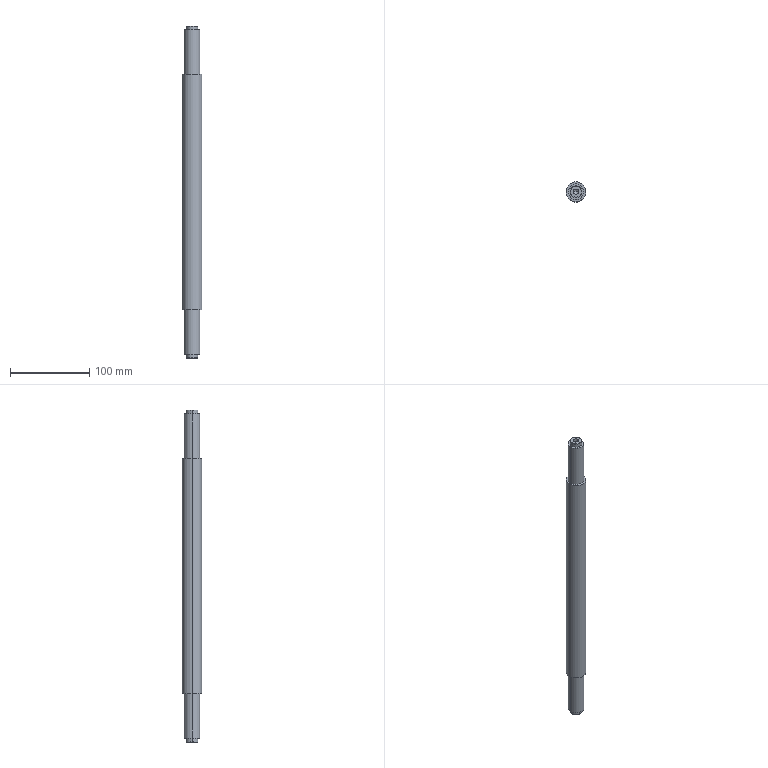Part | SolidWorks | features ICE 4, Chamfer 2, HoleWzd 2, Extrusion 1 | 1 solid | 28 faces | box 25 x 25 x 420 mm | volume 181738 mm3 | cylinder 14 | cone 8 | plane 6 | commonest cylinder face diameters 6.8 x4 15 x4 20 x4 25 x2
STEP:
#1=CARTESIAN_POINT('',(-7.,0.,-61.));
#2=VERTEX_POINT('',#1);
#3=CARTESIAN_POINT('',(7.,0.,-61.));
#4=VERTEX_POINT('',#3);
#5=CARTESIAN_POINT('',(0.,0.,-61.));
#6=DIRECTION('',(0.,0.,-1.));
#7=DIRECTION('',(-1.,0.,0.));
#8=AXIS2_PLACEMENT_3D('',#5,#6,#7);
#9=CIRCLE('',#8,7.);
#10=EDGE_CURVE('',#2,#4,#9,.T.);
#11=ORIENTED_EDGE('',*,*,#10,.F.);
#12=CARTESIAN_POINT('',(-7.5,0.,-60.5));
#13=VERTEX_POINT('',#12);
#14=CARTESIAN_POINT('',(-7.,0.,-61.));
#15=DIRECTION('',(-0.7071,0.,0.7071));
#16=VECTOR('',#15,1000.);
#17=LINE('',#14,#16);
#18=EDGE_CURVE('',#2,#13,#17,.T.);
#19=ORIENTED_EDGE('',*,*,#18,.T.);
#20=CARTESIAN_POINT('',(7.5,0.,-60.5));
#21=VERTEX_POINT('',#20);
#22=CARTESIAN_POINT('',(0.,0.,-60.5));
#23=DIRECTION('',(0.,0.,1.));
#24=DIRECTION('',(-1.,0.,0.));
#25=AXIS2_PLACEMENT_3D('',#22,#23,#24);
#26=CIRCLE('',#25,7.5);
#27=EDGE_CURVE('',#21,#13,#26,.T.);
#28=ORIENTED_EDGE('',*,*,#27,.F.);
#29=CARTESIAN_POINT('',(7.,0.,-61.));
#30=DIRECTION('',(0.7071,0.,0.7071));
#31=VECTOR('',#30,1000.);
#32=LINE('',#29,#31);
#33=EDGE_CURVE('',#4,#21,#32,.T.);
#34=ORIENTED_EDGE('',*,*,#33,.F.);
#35=EDGE_LOOP('',(#11,#19,#28,#34));
#36=FACE_OUTER_BOUND('',#35,.T.);
#37=CARTESIAN_POINT('',(0.,0.,-61.));
#38=DIRECTION('',(0.,0.,1.));
#39=DIRECTION('',(1.,0.,0.));
#40=AXIS2_PLACEMENT_3D('',#37,#38,#39);
#41=CONICAL_SURFACE('',#40,7.,0.7854);
#42=ADVANCED_FACE('',(#36),#41,.T.);
#43=CARTESIAN_POINT('',(7.,0.,359.));
#44=VERTEX_POINT('',#43);
#45=CARTESIAN_POINT('',(-7.,0.,359.));
#46=VERTEX_POINT('',#45);
#47=CARTESIAN_POINT('',(0.,0.,359.));
#48=DIRECTION('',(0.,0.,1.));
#49=DIRECTION('',(1.,0.,0.));
#50=AXIS2_PLACEMENT_3D('',#47,#48,#49);
#51=CIRCLE('',#50,7.);
#52=EDGE_CURVE('',#44,#46,#51,.T.);
#53=ORIENTED_EDGE('',*,*,#52,.F.);
#54=CARTESIAN_POINT('',(7.5,0.,358.5));
#55=VERTEX_POINT('',#54);
#56=CARTESIAN_POINT('',(7.,0.,359.));
#57=DIRECTION('',(0.7071,0.,-0.7071));
#58=VECTOR('',#57,1000.);
#59=LINE('',#56,#58);
#60=EDGE_CURVE('',#44,#55,#59,.T.);
#61=ORIENTED_EDGE('',*,*,#60,.T.);
#62=CARTESIAN_POINT('',(-7.5,0.,358.5));
#63=VERTEX_POINT('',#62);
#64=CARTESIAN_POINT('',(0.,0.,358.5));
#65=DIRECTION('',(0.,0.,-1.));
#66=DIRECTION('',(1.,0.,0.));
#67=AXIS2_PLACEMENT_3D('',#64,#65,#66);
#68=CIRCLE('',#67,7.5);
#69=EDGE_CURVE('',#63,#55,#68,.T.);
#70=ORIENTED_EDGE('',*,*,#69,.F.);
#71=CARTESIAN_POINT('',(-7.,0.,359.));
#72=DIRECTION('',(-0.7071,0.,-0.7071));
#73=VECTOR('',#72,1000.);
#74=LINE('',#71,#73);
#75=EDGE_CURVE('',#46,#63,#74,.T.);
#76=ORIENTED_EDGE('',*,*,#75,.F.);
#77=EDGE_LOOP('',(#53,#61,#70,#76));
#78=FACE_OUTER_BOUND('',#77,.T.);
#79=CARTESIAN_POINT('',(0.,0.,359.));
#80=DIRECTION('',(0.,0.,-1.));
#81=DIRECTION('',(-1.,0.,0.));
#82=AXIS2_PLACEMENT_3D('',#79,#80,#81);
#83=CONICAL_SURFACE('',#82,7.,0.7854);
#84=ADVANCED_FACE('',(#78),#83,.T.);
#85=CARTESIAN_POINT('',(-3.4,0.,339.25));
#86=VERTEX_POINT('',#85);
#87=CARTESIAN_POINT('',(3.4,0.,339.25));
#88=VERTEX_POINT('',#87);
#89=CARTESIAN_POINT('',(0.,0.,339.25));
#90=DIRECTION('',(0.,0.,1.));
#91=DIRECTION('',(1.,0.,0.));
#92=AXIS2_PLACEMENT_3D('',#89,#90,#91);
#93=CIRCLE('',#92,3.4);
#94=EDGE_CURVE('',#86,#88,#93,.T.);
#95=ORIENTED_EDGE('',*,*,#94,.F.);
#96=CARTESIAN_POINT('',(-3.4,0.,359.));
#97=VERTEX_POINT('',#96);
#98=CARTESIAN_POINT('',(-3.4,0.,359.));
#99=DIRECTION('',(0.,0.,1.));
#100=VECTOR('',#99,1000.);
#101=LINE('',#98,#100);
#102=EDGE_CURVE('',#86,#97,#101,.T.);
#103=ORIENTED_EDGE('',*,*,#102,.T.);
#104=CARTESIAN_POINT('',(3.4,0.,359.));
#105=VERTEX_POINT('',#104);
#106=CARTESIAN_POINT('',(0.,0.,359.));
#107=DIRECTION('',(0.,0.,1.));
#108=DIRECTION('',(1.,0.,0.));
#109=AXIS2_PLACEMENT_3D('',#106,#107,#108);
#110=CIRCLE('',#109,3.4);
#111=EDGE_CURVE('',#97,#105,#110,.T.);
#112=ORIENTED_EDGE('',*,*,#111,.T.);
#113=CARTESIAN_POINT('',(3.4,0.,359.));
#114=DIRECTION('',(0.,0.,1.));
#115=VECTOR('',#114,1000.);
#116=LINE('',#113,#115);
#117=EDGE_CURVE('',#88,#105,#116,.T.);
#118=ORIENTED_EDGE('',*,*,#117,.F.);
#119=EDGE_LOOP('',(#95,#103,#112,#118));
#120=FACE_OUTER_BOUND('',#119,.T.);
#121=CARTESIAN_POINT('',(0.,0.,359.));
#122=DIRECTION('',(0.,0.,1.));
#123=DIRECTION('',(1.,0.,0.));
#124=AXIS2_PLACEMENT_3D('',#121,#122,#123);
#125=CYLINDRICAL_SURFACE('',#124,3.4);
#126=ADVANCED_FACE('',(#120),#125,.F.);
#127=CARTESIAN_POINT('',(0.,0.,337.207));
#128=VERTEX_POINT('',#127);
#129=CARTESIAN_POINT('',(3.4,0.,339.25));
#130=DIRECTION('',(0.8572,0.,0.515));
#131=VECTOR('',#130,1000.);
#132=LINE('',#129,#131);
#133=EDGE_CURVE('',#128,#88,#132,.T.);
#134=ORIENTED_EDGE('',*,*,#133,.F.);
#135=CARTESIAN_POINT('',(-3.4,0.,339.25));
#136=DIRECTION('',(-0.8572,0.,0.515));
#137=VECTOR('',#136,1000.);
#138=LINE('',#135,#137);
#139=EDGE_CURVE('',#128,#86,#138,.T.);
#140=ORIENTED_EDGE('',*,*,#139,.T.);
#141=ORIENTED_EDGE('',*,*,#94,.T.);
#142=EDGE_LOOP('',(#134,#140,#141));
#143=FACE_OUTER_BOUND('',#142,.T.);
#144=CARTESIAN_POINT('',(0.,0.,339.25));
#145=DIRECTION('',(0.,0.,1.));
#146=DIRECTION('',(1.,0.,0.));
#147=AXIS2_PLACEMENT_3D('',#144,#145,#146);
#148=CONICAL_SURFACE('',#147,3.4,1.03);
#149=ADVANCED_FACE('',(#143),#148,.F.);
#150=CARTESIAN_POINT('',(3.4,0.,-41.25));
#151=VERTEX_POINT('',#150);
#152=CARTESIAN_POINT('',(-3.4,0.,-41.25));
#153=VERTEX_POINT('',#152);
#154=CARTESIAN_POINT('',(0.,0.,-41.25));
#155=DIRECTION('',(0.,0.,-1.));
#156=DIRECTION('',(-1.,0.,0.));
#157=AXIS2_PLACEMENT_3D('',#154,#155,#156);
#158=CIRCLE('',#157,3.4);
#159=EDGE_CURVE('',#151,#153,#158,.T.);
#160=ORIENTED_EDGE('',*,*,#159,.F.);
#161=CARTESIAN_POINT('',(3.4,0.,-61.));
#162=VERTEX_POINT('',#161);
#163=CARTESIAN_POINT('',(3.4,0.,-61.));
#164=DIRECTION('',(0.,0.,-1.));
#165=VECTOR('',#164,1000.);
#166=LINE('',#163,#165);
#167=EDGE_CURVE('',#151,#162,#166,.T.);
#168=ORIENTED_EDGE('',*,*,#167,.T.);
#169=CARTESIAN_POINT('',(-3.4,0.,-61.));
#170=VERTEX_POINT('',#169);
#171=CARTESIAN_POINT('',(0.,0.,-61.));
#172=DIRECTION('',(0.,0.,-1.));
#173=DIRECTION('',(-1.,0.,0.));
#174=AXIS2_PLACEMENT_3D('',#171,#172,#173);
#175=CIRCLE('',#174,3.4);
#176=EDGE_CURVE('',#162,#170,#175,.T.);
#177=ORIENTED_EDGE('',*,*,#176,.T.);
#178=CARTESIAN_POINT('',(-3.4,0.,-61.));
#179=DIRECTION('',(0.,0.,-1.));
#180=VECTOR('',#179,1000.);
#181=LINE('',#178,#180);
#182=EDGE_CURVE('',#153,#170,#181,.T.);
#183=ORIENTED_EDGE('',*,*,#182,.F.);
#184=EDGE_LOOP('',(#160,#168,#177,#183));
#185=FACE_OUTER_BOUND('',#184,.T.);
#186=CARTESIAN_POINT('',(0.,0.,-61.));
#187=DIRECTION('',(0.,0.,-1.));
#188=DIRECTION('',(-1.,0.,0.));
#189=AXIS2_PLACEMENT_3D('',#186,#187,#188);
#190=CYLINDRICAL_SURFACE('',#189,3.4);
#191=ADVANCED_FACE('',(#185),#190,.F.);
#192=CARTESIAN_POINT('',(0.,0.,-39.207));
#193=VERTEX_POINT('',#192);
#194=CARTESIAN_POINT('',(-3.4,0.,-41.25));
#195=DIRECTION('',(-0.8572,0.,-0.515));
#196=VECTOR('',#195,1000.);
#197=LINE('',#194,#196);
#198=EDGE_CURVE('',#193,#153,#197,.T.);
#199=ORIENTED_EDGE('',*,*,#198,.F.);
#200=CARTESIAN_POINT('',(3.4,0.,-41.25));
#201=DIRECTION('',(0.8572,0.,-0.515));
#202=VECTOR('',#201,1000.);
#203=LINE('',#200,#202);
#204=EDGE_CURVE('',#193,#151,#203,.T.);
#205=ORIENTED_EDGE('',*,*,#204,.T.);
#206=ORIENTED_EDGE('',*,*,#159,.T.);
#207=EDGE_LOOP('',(#199,#205,#206));
#208=FACE_OUTER_BOUND('',#207,.T.);
#209=CARTESIAN_POINT('',(0.,0.,-41.25));
#210=DIRECTION('',(0.,0.,-1.));
#211=DIRECTION('',(-1.,0.,0.));
#212=AXIS2_PLACEMENT_3D('',#209,#210,#211);
#213=CONICAL_SURFACE('',#212,3.4,1.03);
#214=ADVANCED_FACE('',(#208),#213,.F.);
#215=ORIENTED_EDGE('',*,*,#27,.T.);
#216=CARTESIAN_POINT('',(-7.5,0.,-56.));
#217=VERTEX_POINT('',#216);
#218=CARTESIAN_POINT('',(-7.5,0.,-61.));
#219=DIRECTION('',(0.,0.,1.));
#220=VECTOR('',#219,1000.);
#221=LINE('',#218,#220);
#222=EDGE_CURVE('',#13,#217,#221,.T.);
#223=ORIENTED_EDGE('',*,*,#222,.T.);
#224=CARTESIAN_POINT('',(7.5,0.,-56.));
#225=VERTEX_POINT('',#224);
#226=CARTESIAN_POINT('',(0.,0.,-56.));
#227=DIRECTION('',(0.,0.,-1.));
#228=DIRECTION('',(-1.,0.,0.));
#229=AXIS2_PLACEMENT_3D('',#226,#227,#228);
#230=CIRCLE('',#229,7.5);
#231=EDGE_CURVE('',#217,#225,#230,.T.);
#232=ORIENTED_EDGE('',*,*,#231,.T.);
#233=CARTESIAN_POINT('',(7.5,0.,-61.));
#234=DIRECTION('',(0.,0.,1.));
#235=VECTOR('',#234,1000.);
#236=LINE('',#233,#235);
#237=EDGE_CURVE('',#21,#225,#236,.T.);
#238=ORIENTED_EDGE('',*,*,#237,.F.);
#239=EDGE_LOOP('',(#215,#223,#232,#238));
#240=FACE_OUTER_BOUND('',#239,.T.);
#241=CARTESIAN_POINT('',(0.,0.,-61.));
#242=DIRECTION('',(0.,0.,1.));
#243=DIRECTION('',(1.,0.,0.));
#244=AXIS2_PLACEMENT_3D('',#241,#242,#243);
#245=CYLINDRICAL_SURFACE('',#244,7.5);
#246=ADVANCED_FACE('',(#240),#245,.T.);
#247=ORIENTED_EDGE('',*,*,#69,.T.);
#248=CARTESIAN_POINT('',(7.5,0.,354.));
#249=VERTEX_POINT('',#248);
#250=CARTESIAN_POINT('',(7.5,0.,359.));
#251=DIRECTION('',(0.,0.,-1.));
#252=VECTOR('',#251,1000.);
#253=LINE('',#250,#252);
#254=EDGE_CURVE('',#55,#249,#253,.T.);
#255=ORIENTED_EDGE('',*,*,#254,.T.);
#256=CARTESIAN_POINT('',(-7.5,0.,354.));
#257=VERTEX_POINT('',#256);
#258=CARTESIAN_POINT('',(0.,0.,354.));
#259=DIRECTION('',(0.,0.,1.));
#260=DIRECTION('',(1.,0.,0.));
#261=AXIS2_PLACEMENT_3D('',#258,#259,#260);
#262=CIRCLE('',#261,7.5);
#263=EDGE_CURVE('',#249,#257,#262,.T.);
#264=ORIENTED_EDGE('',*,*,#263,.T.);
#265=CARTESIAN_POINT('',(-7.5,0.,359.));
#266=DIRECTION('',(0.,0.,-1.));
#267=VECTOR('',#266,1000.);
#268=LINE('',#265,#267);
#269=EDGE_CURVE('',#63,#257,#268,.T.);
#270=ORIENTED_EDGE('',*,*,#269,.F.);
#271=EDGE_LOOP('',(#247,#255,#264,#270));
#272=FACE_OUTER_BOUND('',#271,.T.);
#273=CARTESIAN_POINT('',(0.,0.,359.));
#274=DIRECTION('',(0.,0.,-1.));
#275=DIRECTION('',(-1.,0.,0.));
#276=AXIS2_PLACEMENT_3D('',#273,#274,#275);
#277=CYLINDRICAL_SURFACE('',#276,7.5);
#278=ADVANCED_FACE('',(#272),#277,.T.);
#279=CARTESIAN_POINT('',(10.,0.,354.));
#280=VERTEX_POINT('',#279);
#281=CARTESIAN_POINT('',(-10.,0.,354.));
#282=VERTEX_POINT('',#281);
#283=CARTESIAN_POINT('',(0.,0.,354.));
#284=DIRECTION('',(0.,0.,1.));
#285=DIRECTION('',(1.,0.,0.));
#286=AXIS2_PLACEMENT_3D('',#283,#284,#285);
#287=CIRCLE('',#286,10.);
#288=EDGE_CURVE('',#280,#282,#287,.T.);
#289=ORIENTED_EDGE('',*,*,#288,.F.);
#290=CARTESIAN_POINT('',(10.,0.,298.));
#291=VERTEX_POINT('',#290);
#292=CARTESIAN_POINT('',(10.,0.,354.));
#293=DIRECTION('',(0.,0.,-1.));
#294=VECTOR('',#293,1000.);
#295=LINE('',#292,#294);
#296=EDGE_CURVE('',#280,#291,#295,.T.);
#297=ORIENTED_EDGE('',*,*,#296,.T.);
#298=CARTESIAN_POINT('',(-10.,0.,298.));
#299=VERTEX_POINT('',#298);
#300=CARTESIAN_POINT('',(0.,0.,298.));
#301=DIRECTION('',(0.,0.,1.));
#302=DIRECTION('',(1.,0.,0.));
#303=AXIS2_PLACEMENT_3D('',#300,#301,#302);
#304=CIRCLE('',#303,10.);
#305=EDGE_CURVE('',#291,#299,#304,.T.);
#306=ORIENTED_EDGE('',*,*,#305,.T.);
#307=CARTESIAN_POINT('',(-10.,0.,354.));
#308=DIRECTION('',(0.,0.,-1.));
#309=VECTOR('',#308,1000.);
#310=LINE('',#307,#309);
#311=EDGE_CURVE('',#282,#299,#310,.T.);
#312=ORIENTED_EDGE('',*,*,#311,.F.);
#313=EDGE_LOOP('',(#289,#297,#306,#312));
#314=FACE_OUTER_BOUND('',#313,.T.);
#315=CARTESIAN_POINT('',(0.,0.,354.));
#316=DIRECTION('',(0.,0.,-1.));
#317=DIRECTION('',(-1.,0.,0.));
#318=AXIS2_PLACEMENT_3D('',#315,#316,#317);
#319=CYLINDRICAL_SURFACE('',#318,10.);
#320=ADVANCED_FACE('',(#314),#319,.T.);
#321=CARTESIAN_POINT('',(-10.,0.,-56.));
#322=VERTEX_POINT('',#321);
#323=CARTESIAN_POINT('',(10.,0.,-56.));
#324=VERTEX_POINT('',#323);
#325=CARTESIAN_POINT('',(0.,0.,-56.));
#326=DIRECTION('',(0.,0.,-1.));
#327=DIRECTION('',(-1.,0.,0.));
#328=AXIS2_PLACEMENT_3D('',#325,#326,#327);
#329=CIRCLE('',#328,10.);
#330=EDGE_CURVE('',#322,#324,#329,.T.);
#331=ORIENTED_EDGE('',*,*,#330,.F.);
#332=CARTESIAN_POINT('',(-10.,0.,0.));
#333=VERTEX_POINT('',#332);
#334=CARTESIAN_POINT('',(-10.,0.,-56.));
#335=DIRECTION('',(0.,0.,1.));
#336=VECTOR('',#335,1000.);
#337=LINE('',#334,#336);
#338=EDGE_CURVE('',#322,#333,#337,.T.);
#339=ORIENTED_EDGE('',*,*,#338,.T.);
#340=CARTESIAN_POINT('',(10.,0.,0.));
#341=VERTEX_POINT('',#340);
#342=CARTESIAN_POINT('',(0.,0.,0.));
#343=DIRECTION('',(0.,0.,-1.));
#344=DIRECTION('',(1.,0.,0.));
#345=AXIS2_PLACEMENT_3D('',#342,#343,#344);
#346=CIRCLE('',#345,10.);
#347=EDGE_CURVE('',#333,#341,#346,.T.);
#348=ORIENTED_EDGE('',*,*,#347,.T.);
#349=CARTESIAN_POINT('',(10.,0.,-56.));
#350=DIRECTION('',(0.,0.,1.));
#351=VECTOR('',#350,1000.);
#352=LINE('',#349,#351);
#353=EDGE_CURVE('',#324,#341,#352,.T.);
#354=ORIENTED_EDGE('',*,*,#353,.F.);
#355=EDGE_LOOP('',(#331,#339,#348,#354));
#356=FACE_OUTER_BOUND('',#355,.T.);
#357=CARTESIAN_POINT('',(0.,0.,-56.));
#358=DIRECTION('',(0.,0.,1.));
#359=DIRECTION('',(1.,0.,0.));
#360=AXIS2_PLACEMENT_3D('',#357,#358,#359);
#361=CYLINDRICAL_SURFACE('',#360,10.);
#362=ADVANCED_FACE('',(#356),#361,.T.);
#363=CARTESIAN_POINT('',(12.5,0.,298.));
#364=VERTEX_POINT('',#363);
#365=CARTESIAN_POINT('',(-12.5,0.,298.));
#366=VERTEX_POINT('',#365);
#367=CARTESIAN_POINT('',(0.,0.,298.));
#368=DIRECTION('',(0.,0.,1.));
#369=DIRECTION('',(1.,0.,0.));
#370=AXIS2_PLACEMENT_3D('',#367,#368,#369);
#371=CIRCLE('',#370,12.5);
#372=EDGE_CURVE('',#364,#366,#371,.T.);
#373=ORIENTED_EDGE('',*,*,#372,.F.);
#374=CARTESIAN_POINT('',(12.5,0.,0.));
#375=VERTEX_POINT('',#374);
#376=CARTESIAN_POINT('',(12.5,0.,298.));
#377=DIRECTION('',(0.,0.,-1.));
#378=VECTOR('',#377,1000.);
#379=LINE('',#376,#378);
#380=EDGE_CURVE('',#364,#375,#379,.T.);
#381=ORIENTED_EDGE('',*,*,#380,.T.);
#382=CARTESIAN_POINT('',(-12.5,0.,0.));
#383=VERTEX_POINT('',#382);
#384=CARTESIAN_POINT('',(0.,0.,0.));
#385=DIRECTION('',(0.,0.,1.));
#386=DIRECTION('',(1.,0.,0.));
#387=AXIS2_PLACEMENT_3D('',#384,#385,#386);
#388=CIRCLE('',#387,12.5);
#389=EDGE_CURVE('',#375,#383,#388,.T.);
#390=ORIENTED_EDGE('',*,*,#389,.T.);
#391=CARTESIAN_POINT('',(-12.5,0.,298.));
#392=DIRECTION('',(0.,0.,-1.));
#393=VECTOR('',#392,1000.);
#394=LINE('',#391,#393);
#395=EDGE_CURVE('',#366,#383,#394,.T.);
#396=ORIENTED_EDGE('',*,*,#395,.F.);
#397=EDGE_LOOP('',(#373,#381,#390,#396));
#398=FACE_OUTER_BOUND('',#397,.T.);
#399=CARTESIAN_POINT('',(0.,0.,298.));
#400=DIRECTION('',(0.,0.,-1.));
#401=DIRECTION('',(-1.,0.,0.));
#402=AXIS2_PLACEMENT_3D('',#399,#400,#401);
#403=CYLINDRICAL_SURFACE('',#402,12.5);
#404=ADVANCED_FACE('',(#398),#403,.T.);
#405=CARTESIAN_POINT('',(0.,0.,-56.));
#406=DIRECTION('',(0.,0.,-1.));
#407=DIRECTION('',(-1.,0.,0.));
#408=AXIS2_PLACEMENT_3D('',#405,#406,#407);
#409=CIRCLE('',#408,10.);
#410=EDGE_CURVE('',#324,#322,#409,.T.);
#411=ORIENTED_EDGE('',*,*,#410,.T.);
#412=ORIENTED_EDGE('',*,*,#330,.T.);
#413=EDGE_LOOP('',(#411,#412));
#414=FACE_OUTER_BOUND('',#413,.T.);
#415=CARTESIAN_POINT('',(0.,0.,-56.));
#416=DIRECTION('',(0.,0.,-1.));
#417=DIRECTION('',(-1.,0.,0.));
#418=AXIS2_PLACEMENT_3D('',#415,#416,#417);
#419=CIRCLE('',#418,7.5);
#420=EDGE_CURVE('',#225,#217,#419,.T.);
#421=ORIENTED_EDGE('',*,*,#420,.F.);
#422=ORIENTED_EDGE('',*,*,#231,.F.);
#423=EDGE_LOOP('',(#421,#422));
#424=FACE_BOUND('',#423,.T.);
#425=CARTESIAN_POINT('',(0.,0.,-56.));
#426=DIRECTION('',(0.,0.,-1.));
#427=DIRECTION('',(-1.,0.,0.));
#428=AXIS2_PLACEMENT_3D('',#425,#426,#427);
#429=PLANE('',#428);
#430=ADVANCED_FACE('',(#414,#424),#429,.T.);
#431=CARTESIAN_POINT('',(0.,0.,354.));
#432=DIRECTION('',(0.,0.,1.));
#433=DIRECTION('',(1.,0.,0.));
#434=AXIS2_PLACEMENT_3D('',#431,#432,#433);
#435=CIRCLE('',#434,10.);
#436=EDGE_CURVE('',#282,#280,#435,.T.);
#437=ORIENTED_EDGE('',*,*,#436,.T.);
#438=ORIENTED_EDGE('',*,*,#288,.T.);
#439=EDGE_LOOP('',(#437,#438));
#440=FACE_OUTER_BOUND('',#439,.T.);
#441=CARTESIAN_POINT('',(0.,0.,354.));
#442=DIRECTION('',(0.,0.,1.));
#443=DIRECTION('',(1.,0.,0.));
#444=AXIS2_PLACEMENT_3D('',#441,#442,#443);
#445=CIRCLE('',#444,7.5);
#446=EDGE_CURVE('',#257,#249,#445,.T.);
#447=ORIENTED_EDGE('',*,*,#446,.F.);
#448=ORIENTED_EDGE('',*,*,#263,.F.);
#449=EDGE_LOOP('',(#447,#448));
#450=FACE_BOUND('',#449,.T.);
#451=CARTESIAN_POINT('',(0.,0.,354.));
#452=DIRECTION('',(0.,0.,1.));
#453=DIRECTION('',(1.,0.,0.));
#454=AXIS2_PLACEMENT_3D('',#451,#452,#453);
#455=PLANE('',#454);
#456=ADVANCED_FACE('',(#440,#450),#455,.T.);
#457=CARTESIAN_POINT('',(0.,0.,298.));
#458=DIRECTION('',(0.,0.,1.));
#459=DIRECTION('',(1.,0.,0.));
#460=AXIS2_PLACEMENT_3D('',#457,#458,#459);
#461=CIRCLE('',#460,12.5);
#462=EDGE_CURVE('',#366,#364,#461,.T.);
#463=ORIENTED_EDGE('',*,*,#462,.T.);
#464=ORIENTED_EDGE('',*,*,#372,.T.);
#465=EDGE_LOOP('',(#463,#464));
#466=FACE_OUTER_BOUND('',#465,.T.);
#467=CARTESIAN_POINT('',(0.,0.,298.));
#468=DIRECTION('',(0.,0.,1.));
#469=DIRECTION('',(1.,0.,0.));
#470=AXIS2_PLACEMENT_3D('',#467,#468,#469);
#471=CIRCLE('',#470,10.);
#472=EDGE_CURVE('',#299,#291,#471,.T.);
#473=ORIENTED_EDGE('',*,*,#472,.F.);
#474=ORIENTED_EDGE('',*,*,#305,.F.);
#475=EDGE_LOOP('',(#473,#474));
#476=FACE_BOUND('',#475,.T.);
#477=CARTESIAN_POINT('',(0.,0.,298.));
#478=DIRECTION('',(0.,0.,1.));
#479=DIRECTION('',(1.,0.,0.));
#480=AXIS2_PLACEMENT_3D('',#477,#478,#479);
#481=PLANE('',#480);
#482=ADVANCED_FACE('',(#466,#476),#481,.T.);
#483=CARTESIAN_POINT('',(0.,0.,0.));
#484=DIRECTION('',(0.,0.,1.));
#485=DIRECTION('',(1.,0.,0.));
#486=AXIS2_PLACEMENT_3D('',#483,#484,#485);
#487=CIRCLE('',#486,12.5);
#488=EDGE_CURVE('',#383,#375,#487,.T.);
#489=ORIENTED_EDGE('',*,*,#488,.F.);
#490=ORIENTED_EDGE('',*,*,#389,.F.);
#491=EDGE_LOOP('',(#489,#490));
#492=FACE_OUTER_BOUND('',#491,.T.);
#493=CARTESIAN_POINT('',(0.,0.,0.));
#494=DIRECTION('',(0.,0.,-1.));
#495=DIRECTION('',(1.,0.,0.));
#496=AXIS2_PLACEMENT_3D('',#493,#494,#495);
#497=CIRCLE('',#496,10.);
#498=EDGE_CURVE('',#341,#333,#497,.T.);
#499=ORIENTED_EDGE('',*,*,#498,.F.);
#500=ORIENTED_EDGE('',*,*,#347,.F.);
#501=EDGE_LOOP('',(#499,#500));
#502=FACE_BOUND('',#501,.T.);
#503=CARTESIAN_POINT('',(0.,0.,0.));
#504=DIRECTION('',(0.,0.,1.));
#505=DIRECTION('',(1.,0.,0.));
#506=AXIS2_PLACEMENT_3D('',#503,#504,#505);
#507=PLANE('',#506);
#508=ADVANCED_FACE('',(#492,#502),#507,.F.);
#509=ORIENTED_EDGE('',*,*,#380,.F.);
#510=ORIENTED_EDGE('',*,*,#462,.F.);
#511=ORIENTED_EDGE('',*,*,#395,.T.);
#512=ORIENTED_EDGE('',*,*,#488,.T.);
#513=EDGE_LOOP('',(#509,#510,#511,#512));
#514=FACE_OUTER_BOUND('',#513,.T.);
#515=CARTESIAN_POINT('',(0.,0.,298.));
#516=DIRECTION('',(0.,0.,-1.));
#517=DIRECTION('',(-1.,0.,0.));
#518=AXIS2_PLACEMENT_3D('',#515,#516,#517);
#519=CYLINDRICAL_SURFACE('',#518,12.5);
#520=ADVANCED_FACE('',(#514),#519,.T.);
#521=ORIENTED_EDGE('',*,*,#338,.F.);
#522=ORIENTED_EDGE('',*,*,#410,.F.);
#523=ORIENTED_EDGE('',*,*,#353,.T.);
#524=ORIENTED_EDGE('',*,*,#498,.T.);
#525=EDGE_LOOP('',(#521,#522,#523,#524));
#526=FACE_OUTER_BOUND('',#525,.T.);
#527=CARTESIAN_POINT('',(0.,0.,-56.));
#528=DIRECTION('',(0.,0.,1.));
#529=DIRECTION('',(1.,0.,0.));
#530=AXIS2_PLACEMENT_3D('',#527,#528,#529);
#531=CYLINDRICAL_SURFACE('',#530,10.);
#532=ADVANCED_FACE('',(#526),#531,.T.);
#533=ORIENTED_EDGE('',*,*,#296,.F.);
#534=ORIENTED_EDGE('',*,*,#436,.F.);
#535=ORIENTED_EDGE('',*,*,#311,.T.);
#536=ORIENTED_EDGE('',*,*,#472,.T.);
#537=EDGE_LOOP('',(#533,#534,#535,#536));
#538=FACE_OUTER_BOUND('',#537,.T.);
#539=CARTESIAN_POINT('',(0.,0.,354.));
#540=DIRECTION('',(0.,0.,-1.));
#541=DIRECTION('',(-1.,0.,0.));
#542=AXIS2_PLACEMENT_3D('',#539,#540,#541);
#543=CYLINDRICAL_SURFACE('',#542,10.);
#544=ADVANCED_FACE('',(#538),#543,.T.);
#545=ORIENTED_EDGE('',*,*,#254,.F.);
#546=CARTESIAN_POINT('',(0.,0.,358.5));
#547=DIRECTION('',(0.,0.,-1.));
#548=DIRECTION('',(1.,0.,0.));
#549=AXIS2_PLACEMENT_3D('',#546,#547,#548);
#550=CIRCLE('',#549,7.5);
#551=EDGE_CURVE('',#55,#63,#550,.T.);
#552=ORIENTED_EDGE('',*,*,#551,.T.);
#553=ORIENTED_EDGE('',*,*,#269,.T.);
#554=ORIENTED_EDGE('',*,*,#446,.T.);
#555=EDGE_LOOP('',(#545,#552,#553,#554));
#556=FACE_OUTER_BOUND('',#555,.T.);
#557=CARTESIAN_POINT('',(0.,0.,359.));
#558=DIRECTION('',(0.,0.,-1.));
#559=DIRECTION('',(-1.,0.,0.));
#560=AXIS2_PLACEMENT_3D('',#557,#558,#559);
#561=CYLINDRICAL_SURFACE('',#560,7.5);
#562=ADVANCED_FACE('',(#556),#561,.T.);
#563=CARTESIAN_POINT('',(0.,0.,359.));
#564=DIRECTION('',(0.,0.,1.));
#565=DIRECTION('',(1.,0.,0.));
#566=AXIS2_PLACEMENT_3D('',#563,#564,#565);
#567=CIRCLE('',#566,7.);
#568=EDGE_CURVE('',#46,#44,#567,.T.);
#569=ORIENTED_EDGE('',*,*,#568,.T.);
#570=ORIENTED_EDGE('',*,*,#52,.T.);
#571=EDGE_LOOP('',(#569,#570));
#572=FACE_OUTER_BOUND('',#571,.T.);
#573=CARTESIAN_POINT('',(0.,0.,359.));
#574=DIRECTION('',(0.,0.,1.));
#575=DIRECTION('',(1.,0.,0.));
#576=AXIS2_PLACEMENT_3D('',#573,#574,#575);
#577=CIRCLE('',#576,3.4);
#578=EDGE_CURVE('',#105,#97,#577,.T.);
#579=ORIENTED_EDGE('',*,*,#578,.F.);
#580=ORIENTED_EDGE('',*,*,#111,.F.);
#581=EDGE_LOOP('',(#579,#580));
#582=FACE_BOUND('',#581,.T.);
#583=CARTESIAN_POINT('',(0.,0.,359.));
#584=DIRECTION('',(0.,0.,1.));
#585=DIRECTION('',(1.,0.,0.));
#586=AXIS2_PLACEMENT_3D('',#583,#584,#585);
#587=PLANE('',#586);
#588=ADVANCED_FACE('',(#572,#582),#587,.T.);
#589=ORIENTED_EDGE('',*,*,#222,.F.);
#590=CARTESIAN_POINT('',(0.,0.,-60.5));
#591=DIRECTION('',(0.,0.,1.));
#592=DIRECTION('',(-1.,0.,0.));
#593=AXIS2_PLACEMENT_3D('',#590,#591,#592);
#594=CIRCLE('',#593,7.5);
#595=EDGE_CURVE('',#13,#21,#594,.T.);
#596=ORIENTED_EDGE('',*,*,#595,.T.);
#597=ORIENTED_EDGE('',*,*,#237,.T.);
#598=ORIENTED_EDGE('',*,*,#420,.T.);
#599=EDGE_LOOP('',(#589,#596,#597,#598));
#600=FACE_OUTER_BOUND('',#599,.T.);
#601=CARTESIAN_POINT('',(0.,0.,-61.));
#602=DIRECTION('',(0.,0.,1.));
#603=DIRECTION('',(1.,0.,0.));
#604=AXIS2_PLACEMENT_3D('',#601,#602,#603);
#605=CYLINDRICAL_SURFACE('',#604,7.5);
#606=ADVANCED_FACE('',(#600),#605,.T.);
#607=CARTESIAN_POINT('',(0.,0.,-61.));
#608=DIRECTION('',(0.,0.,-1.));
#609=DIRECTION('',(-1.,0.,0.));
#610=AXIS2_PLACEMENT_3D('',#607,#608,#609);
#611=CIRCLE('',#610,7.);
#612=EDGE_CURVE('',#4,#2,#611,.T.);
#613=ORIENTED_EDGE('',*,*,#612,.T.);
#614=ORIENTED_EDGE('',*,*,#10,.T.);
#615=EDGE_LOOP('',(#613,#614));
#616=FACE_OUTER_BOUND('',#615,.T.);
#617=CARTESIAN_POINT('',(0.,0.,-61.));
#618=DIRECTION('',(0.,0.,-1.));
#619=DIRECTION('',(-1.,0.,0.));
#620=AXIS2_PLACEMENT_3D('',#617,#618,#619);
#621=CIRCLE('',#620,3.4);
#622=EDGE_CURVE('',#170,#162,#621,.T.);
#623=ORIENTED_EDGE('',*,*,#622,.F.);
#624=ORIENTED_EDGE('',*,*,#176,.F.);
#625=EDGE_LOOP('',(#623,#624));
#626=FACE_BOUND('',#625,.T.);
#627=CARTESIAN_POINT('',(0.,0.,-61.));
#628=DIRECTION('',(0.,0.,-1.));
#629=DIRECTION('',(-1.,0.,0.));
#630=AXIS2_PLACEMENT_3D('',#627,#628,#629);
#631=PLANE('',#630);
#632=ADVANCED_FACE('',(#616,#626),#631,.T.);
#633=ORIENTED_EDGE('',*,*,#204,.F.);
#634=ORIENTED_EDGE('',*,*,#198,.T.);
#635=CARTESIAN_POINT('',(0.,0.,-41.25));
#636=DIRECTION('',(0.,0.,-1.));
#637=DIRECTION('',(-1.,0.,0.));
#638=AXIS2_PLACEMENT_3D('',#635,#636,#637);
#639=CIRCLE('',#638,3.4);
#640=EDGE_CURVE('',#153,#151,#639,.T.);
#641=ORIENTED_EDGE('',*,*,#640,.T.);
#642=EDGE_LOOP('',(#633,#634,#641));
#643=FACE_OUTER_BOUND('',#642,.T.);
#644=CARTESIAN_POINT('',(0.,0.,-41.25));
#645=DIRECTION('',(0.,0.,-1.));
#646=DIRECTION('',(-1.,0.,0.));
#647=AXIS2_PLACEMENT_3D('',#644,#645,#646);
#648=CONICAL_SURFACE('',#647,3.4,1.03);
#649=ADVANCED_FACE('',(#643),#648,.F.);
#650=ORIENTED_EDGE('',*,*,#167,.F.);
#651=ORIENTED_EDGE('',*,*,#640,.F.);
#652=ORIENTED_EDGE('',*,*,#182,.T.);
#653=ORIENTED_EDGE('',*,*,#622,.T.);
#654=EDGE_LOOP('',(#650,#651,#652,#653));
#655=FACE_OUTER_BOUND('',#654,.T.);
#656=CARTESIAN_POINT('',(0.,0.,-61.));
#657=DIRECTION('',(0.,0.,-1.));
#658=DIRECTION('',(-1.,0.,0.));
#659=AXIS2_PLACEMENT_3D('',#656,#657,#658);
#660=CYLINDRICAL_SURFACE('',#659,3.4);
#661=ADVANCED_FACE('',(#655),#660,.F.);
#662=ORIENTED_EDGE('',*,*,#139,.F.);
#663=ORIENTED_EDGE('',*,*,#133,.T.);
#664=CARTESIAN_POINT('',(0.,0.,339.25));
#665=DIRECTION('',(0.,0.,1.));
#666=DIRECTION('',(1.,0.,0.));
#667=AXIS2_PLACEMENT_3D('',#664,#665,#666);
#668=CIRCLE('',#667,3.4);
#669=EDGE_CURVE('',#88,#86,#668,.T.);
#670=ORIENTED_EDGE('',*,*,#669,.T.);
#671=EDGE_LOOP('',(#662,#663,#670));
#672=FACE_OUTER_BOUND('',#671,.T.);
#673=CARTESIAN_POINT('',(0.,0.,339.25));
#674=DIRECTION('',(0.,0.,1.));
#675=DIRECTION('',(1.,0.,0.));
#676=AXIS2_PLACEMENT_3D('',#673,#674,#675);
#677=CONICAL_SURFACE('',#676,3.4,1.03);
#678=ADVANCED_FACE('',(#672),#677,.F.);
#679=ORIENTED_EDGE('',*,*,#102,.F.);
#680=ORIENTED_EDGE('',*,*,#669,.F.);
#681=ORIENTED_EDGE('',*,*,#117,.T.);
#682=ORIENTED_EDGE('',*,*,#578,.T.);
#683=EDGE_LOOP('',(#679,#680,#681,#682));
#684=FACE_OUTER_BOUND('',#683,.T.);
#685=CARTESIAN_POINT('',(0.,0.,359.));
#686=DIRECTION('',(0.,0.,1.));
#687=DIRECTION('',(1.,0.,0.));
#688=AXIS2_PLACEMENT_3D('',#685,#686,#687);
#689=CYLINDRICAL_SURFACE('',#688,3.4);
#690=ADVANCED_FACE('',(#684),#689,.F.);
#691=ORIENTED_EDGE('',*,*,#60,.F.);
#692=ORIENTED_EDGE('',*,*,#568,.F.);
#693=ORIENTED_EDGE('',*,*,#75,.T.);
#694=ORIENTED_EDGE('',*,*,#551,.F.);
#695=EDGE_LOOP('',(#691,#692,#693,#694));
#696=FACE_OUTER_BOUND('',#695,.T.);
#697=CARTESIAN_POINT('',(0.,0.,359.));
#698=DIRECTION('',(0.,0.,-1.));
#699=DIRECTION('',(-1.,0.,0.));
#700=AXIS2_PLACEMENT_3D('',#697,#698,#699);
#701=CONICAL_SURFACE('',#700,7.,0.7854);
#702=ADVANCED_FACE('',(#696),#701,.T.);
#703=ORIENTED_EDGE('',*,*,#18,.F.);
#704=ORIENTED_EDGE('',*,*,#612,.F.);
#705=ORIENTED_EDGE('',*,*,#33,.T.);
#706=ORIENTED_EDGE('',*,*,#595,.F.);
#707=EDGE_LOOP('',(#703,#704,#705,#706));
#708=FACE_OUTER_BOUND('',#707,.T.);
#709=CARTESIAN_POINT('',(0.,0.,-61.));
#710=DIRECTION('',(0.,0.,1.));
#711=DIRECTION('',(1.,0.,0.));
#712=AXIS2_PLACEMENT_3D('',#709,#710,#711);
#713=CONICAL_SURFACE('',#712,7.,0.7854);
#714=ADVANCED_FACE('',(#708),#713,.T.);
#715=CLOSED_SHELL('',(#42,#84,#126,#149,#191,#214,#246,#278,#320,#362,#404,#430,#456,#482,#508,#520,#532,#544,#562,#588,#606,#632,#649,#661,#678,#690,#702,#714));
#716=MANIFOLD_SOLID_BREP('',#715);
#717=CARTESIAN_POINT('',(0.,0.,0.));
#718=DIRECTION('',(0.,0.,1.));
#719=DIRECTION('',(1.,0.,0.));
#720=AXIS2_PLACEMENT_3D('',#717,#718,#719);
#721=(LENGTH_UNIT()NAMED_UNIT(*)SI_UNIT(.MILLI.,.METRE.));
#722=UNCERTAINTY_MEASURE_WITH_UNIT(LENGTH_MEASURE(0.00001),#721,'','');
#723=(NAMED_UNIT(*)PLANE_ANGLE_UNIT()SI_UNIT($,.RADIAN.));
#724=(NAMED_UNIT(*)SI_UNIT($,.STERADIAN.)SOLID_ANGLE_UNIT());
#725=(GEOMETRIC_REPRESENTATION_CONTEXT(3)GLOBAL_UNCERTAINTY_ASSIGNED_CONTEXT((#722))GLOBAL_UNIT_ASSIGNED_CONTEXT((#721,#723,#724))REPRESENTATION_CONTEXT('',''));
#726=ADVANCED_BREP_SHAPE_REPRESENTATION('',(#716,#720),#725);